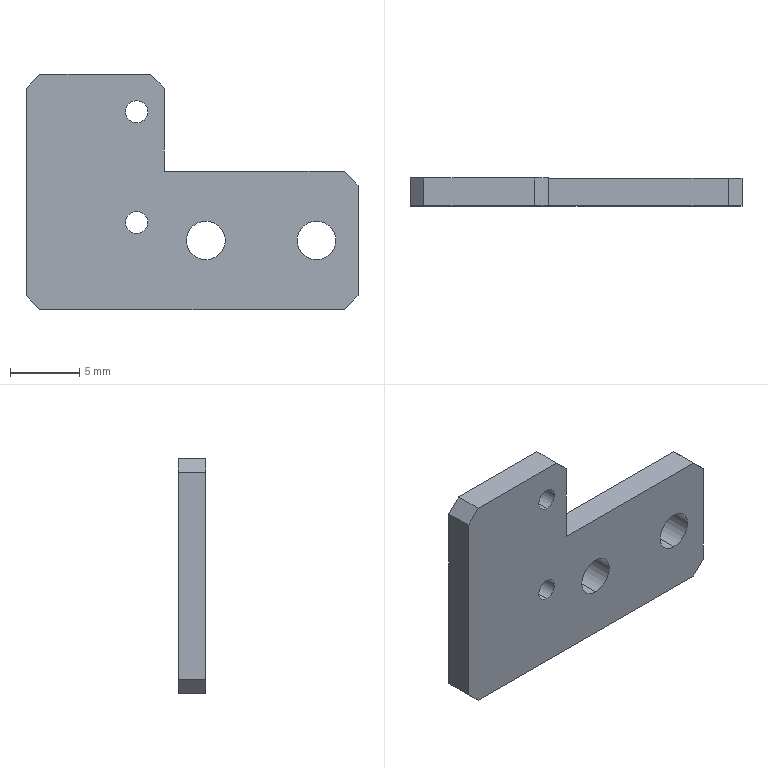Part | SolidWorks | features ICE 2, Chamfer 1, Extrusion 1, HoleWzd 1 | 1 solid | 21 faces | box 24 x 2 x 17 mm | volume 582.327 mm3 | plane 13 | cylinder 8 | commonest cylinder face diameters 1.6 x4 2.8 x4
STEP:
#1=CARTESIAN_POINT('',(8.,0.,-9.9));
#2=VERTEX_POINT('',#1);
#3=CARTESIAN_POINT('',(8.,0.,-11.5));
#4=VERTEX_POINT('',#3);
#5=CARTESIAN_POINT('',(8.,0.,-10.7));
#6=DIRECTION('',(0.,-1.,0.));
#7=DIRECTION('',(0.,0.,-1.));
#8=AXIS2_PLACEMENT_3D('',#5,#6,#7);
#9=CIRCLE('',#8,0.8);
#10=EDGE_CURVE('',#2,#4,#9,.T.);
#11=ORIENTED_EDGE('',*,*,#10,.T.);
#12=CARTESIAN_POINT('',(8.,2.,-11.5));
#13=VERTEX_POINT('',#12);
#14=CARTESIAN_POINT('',(8.,2.,-11.5));
#15=DIRECTION('',(0.,1.,0.));
#16=VECTOR('',#15,1000.);
#17=LINE('',#14,#16);
#18=EDGE_CURVE('',#4,#13,#17,.T.);
#19=ORIENTED_EDGE('',*,*,#18,.T.);
#20=CARTESIAN_POINT('',(8.,2.,-9.9));
#21=VERTEX_POINT('',#20);
#22=CARTESIAN_POINT('',(8.,2.,-10.7));
#23=DIRECTION('',(0.,1.,0.));
#24=DIRECTION('',(0.,0.,1.));
#25=AXIS2_PLACEMENT_3D('',#22,#23,#24);
#26=CIRCLE('',#25,0.8);
#27=EDGE_CURVE('',#13,#21,#26,.T.);
#28=ORIENTED_EDGE('',*,*,#27,.T.);
#29=CARTESIAN_POINT('',(8.,2.,-9.9));
#30=DIRECTION('',(0.,1.,0.));
#31=VECTOR('',#30,1000.);
#32=LINE('',#29,#31);
#33=EDGE_CURVE('',#2,#21,#32,.T.);
#34=ORIENTED_EDGE('',*,*,#33,.F.);
#35=EDGE_LOOP('',(#11,#19,#28,#34));
#36=FACE_OUTER_BOUND('',#35,.T.);
#37=CARTESIAN_POINT('',(8.,2.,-10.7));
#38=DIRECTION('',(0.,1.,0.));
#39=DIRECTION('',(0.,0.,1.));
#40=AXIS2_PLACEMENT_3D('',#37,#38,#39);
#41=CYLINDRICAL_SURFACE('',#40,0.8);
#42=ADVANCED_FACE('',(#36),#41,.F.);
#43=CARTESIAN_POINT('',(8.,0.,-1.9));
#44=VERTEX_POINT('',#43);
#45=CARTESIAN_POINT('',(8.,0.,-3.5));
#46=VERTEX_POINT('',#45);
#47=CARTESIAN_POINT('',(8.,0.,-2.7));
#48=DIRECTION('',(0.,-1.,0.));
#49=DIRECTION('',(0.,0.,-1.));
#50=AXIS2_PLACEMENT_3D('',#47,#48,#49);
#51=CIRCLE('',#50,0.8);
#52=EDGE_CURVE('',#44,#46,#51,.T.);
#53=ORIENTED_EDGE('',*,*,#52,.T.);
#54=CARTESIAN_POINT('',(8.,2.,-3.5));
#55=VERTEX_POINT('',#54);
#56=CARTESIAN_POINT('',(8.,2.,-3.5));
#57=DIRECTION('',(0.,1.,0.));
#58=VECTOR('',#57,1000.);
#59=LINE('',#56,#58);
#60=EDGE_CURVE('',#46,#55,#59,.T.);
#61=ORIENTED_EDGE('',*,*,#60,.T.);
#62=CARTESIAN_POINT('',(8.,2.,-1.9));
#63=VERTEX_POINT('',#62);
#64=CARTESIAN_POINT('',(8.,2.,-2.7));
#65=DIRECTION('',(0.,1.,0.));
#66=DIRECTION('',(0.,0.,1.));
#67=AXIS2_PLACEMENT_3D('',#64,#65,#66);
#68=CIRCLE('',#67,0.8);
#69=EDGE_CURVE('',#55,#63,#68,.T.);
#70=ORIENTED_EDGE('',*,*,#69,.T.);
#71=CARTESIAN_POINT('',(8.,2.,-1.9));
#72=DIRECTION('',(0.,1.,0.));
#73=VECTOR('',#72,1000.);
#74=LINE('',#71,#73);
#75=EDGE_CURVE('',#44,#63,#74,.T.);
#76=ORIENTED_EDGE('',*,*,#75,.F.);
#77=EDGE_LOOP('',(#53,#61,#70,#76));
#78=FACE_OUTER_BOUND('',#77,.T.);
#79=CARTESIAN_POINT('',(8.,2.,-2.7));
#80=DIRECTION('',(0.,1.,0.));
#81=DIRECTION('',(0.,0.,1.));
#82=AXIS2_PLACEMENT_3D('',#79,#80,#81);
#83=CYLINDRICAL_SURFACE('',#82,0.8);
#84=ADVANCED_FACE('',(#78),#83,.F.);
#85=CARTESIAN_POINT('',(13.,0.,-10.6));
#86=VERTEX_POINT('',#85);
#87=CARTESIAN_POINT('',(13.,0.,-13.4));
#88=VERTEX_POINT('',#87);
#89=CARTESIAN_POINT('',(13.,0.,-12.));
#90=DIRECTION('',(0.,-1.,0.));
#91=DIRECTION('',(0.,0.,-1.));
#92=AXIS2_PLACEMENT_3D('',#89,#90,#91);
#93=CIRCLE('',#92,1.4);
#94=EDGE_CURVE('',#86,#88,#93,.T.);
#95=ORIENTED_EDGE('',*,*,#94,.T.);
#96=CARTESIAN_POINT('',(13.,2.,-13.4));
#97=VERTEX_POINT('',#96);
#98=CARTESIAN_POINT('',(13.,-8.,-13.4));
#99=DIRECTION('',(0.,1.,0.));
#100=VECTOR('',#99,1000.);
#101=LINE('',#98,#100);
#102=EDGE_CURVE('',#88,#97,#101,.T.);
#103=ORIENTED_EDGE('',*,*,#102,.T.);
#104=CARTESIAN_POINT('',(13.,2.,-10.6));
#105=VERTEX_POINT('',#104);
#106=CARTESIAN_POINT('',(13.,2.,-12.));
#107=DIRECTION('',(0.,1.,0.));
#108=DIRECTION('',(0.,0.,1.));
#109=AXIS2_PLACEMENT_3D('',#106,#107,#108);
#110=CIRCLE('',#109,1.4);
#111=EDGE_CURVE('',#97,#105,#110,.T.);
#112=ORIENTED_EDGE('',*,*,#111,.T.);
#113=CARTESIAN_POINT('',(13.,-8.,-10.6));
#114=DIRECTION('',(0.,1.,0.));
#115=VECTOR('',#114,1000.);
#116=LINE('',#113,#115);
#117=EDGE_CURVE('',#86,#105,#116,.T.);
#118=ORIENTED_EDGE('',*,*,#117,.F.);
#119=EDGE_LOOP('',(#95,#103,#112,#118));
#120=FACE_OUTER_BOUND('',#119,.T.);
#121=CARTESIAN_POINT('',(13.,-8.,-12.));
#122=DIRECTION('',(0.,1.,0.));
#123=DIRECTION('',(0.,0.,1.));
#124=AXIS2_PLACEMENT_3D('',#121,#122,#123);
#125=CYLINDRICAL_SURFACE('',#124,1.4);
#126=ADVANCED_FACE('',(#120),#125,.F.);
#127=CARTESIAN_POINT('',(21.,0.,-10.6));
#128=VERTEX_POINT('',#127);
#129=CARTESIAN_POINT('',(21.,0.,-13.4));
#130=VERTEX_POINT('',#129);
#131=CARTESIAN_POINT('',(21.,0.,-12.));
#132=DIRECTION('',(0.,-1.,0.));
#133=DIRECTION('',(0.,0.,-1.));
#134=AXIS2_PLACEMENT_3D('',#131,#132,#133);
#135=CIRCLE('',#134,1.4);
#136=EDGE_CURVE('',#128,#130,#135,.T.);
#137=ORIENTED_EDGE('',*,*,#136,.T.);
#138=CARTESIAN_POINT('',(21.,2.,-13.4));
#139=VERTEX_POINT('',#138);
#140=CARTESIAN_POINT('',(21.,-8.,-13.4));
#141=DIRECTION('',(0.,1.,0.));
#142=VECTOR('',#141,1000.);
#143=LINE('',#140,#142);
#144=EDGE_CURVE('',#130,#139,#143,.T.);
#145=ORIENTED_EDGE('',*,*,#144,.T.);
#146=CARTESIAN_POINT('',(21.,2.,-10.6));
#147=VERTEX_POINT('',#146);
#148=CARTESIAN_POINT('',(21.,2.,-12.));
#149=DIRECTION('',(0.,1.,0.));
#150=DIRECTION('',(0.,0.,1.));
#151=AXIS2_PLACEMENT_3D('',#148,#149,#150);
#152=CIRCLE('',#151,1.4);
#153=EDGE_CURVE('',#139,#147,#152,.T.);
#154=ORIENTED_EDGE('',*,*,#153,.T.);
#155=CARTESIAN_POINT('',(21.,-8.,-10.6));
#156=DIRECTION('',(0.,1.,0.));
#157=VECTOR('',#156,1000.);
#158=LINE('',#155,#157);
#159=EDGE_CURVE('',#128,#147,#158,.T.);
#160=ORIENTED_EDGE('',*,*,#159,.F.);
#161=EDGE_LOOP('',(#137,#145,#154,#160));
#162=FACE_OUTER_BOUND('',#161,.T.);
#163=CARTESIAN_POINT('',(21.,-8.,-12.));
#164=DIRECTION('',(0.,1.,0.));
#165=DIRECTION('',(0.,0.,1.));
#166=AXIS2_PLACEMENT_3D('',#163,#164,#165);
#167=CYLINDRICAL_SURFACE('',#166,1.4);
#168=ADVANCED_FACE('',(#162),#167,.F.);
#169=CARTESIAN_POINT('',(0.,2.,-16.));
#170=VERTEX_POINT('',#169);
#171=CARTESIAN_POINT('',(0.,2.,-1.));
#172=VERTEX_POINT('',#171);
#173=CARTESIAN_POINT('',(0.,2.,0.));
#174=DIRECTION('',(0.,0.,1.));
#175=VECTOR('',#174,1000.);
#176=LINE('',#173,#175);
#177=EDGE_CURVE('',#170,#172,#176,.T.);
#178=ORIENTED_EDGE('',*,*,#177,.F.);
#179=CARTESIAN_POINT('',(0.,0.,-16.));
#180=VERTEX_POINT('',#179);
#181=CARTESIAN_POINT('',(0.,2.,-16.));
#182=DIRECTION('',(0.,-1.,0.));
#183=VECTOR('',#182,1000.);
#184=LINE('',#181,#183);
#185=EDGE_CURVE('',#170,#180,#184,.T.);
#186=ORIENTED_EDGE('',*,*,#185,.T.);
#187=CARTESIAN_POINT('',(0.,0.,-1.));
#188=VERTEX_POINT('',#187);
#189=CARTESIAN_POINT('',(0.,0.,0.));
#190=DIRECTION('',(0.,0.,1.));
#191=VECTOR('',#190,1000.);
#192=LINE('',#189,#191);
#193=EDGE_CURVE('',#180,#188,#192,.T.);
#194=ORIENTED_EDGE('',*,*,#193,.T.);
#195=CARTESIAN_POINT('',(0.,2.,-1.));
#196=DIRECTION('',(0.,1.,0.));
#197=VECTOR('',#196,1000.);
#198=LINE('',#195,#197);
#199=EDGE_CURVE('',#188,#172,#198,.T.);
#200=ORIENTED_EDGE('',*,*,#199,.T.);
#201=EDGE_LOOP('',(#178,#186,#194,#200));
#202=FACE_OUTER_BOUND('',#201,.T.);
#203=CARTESIAN_POINT('',(0.,2.,0.));
#204=DIRECTION('',(1.,0.,0.));
#205=DIRECTION('',(0.,0.,-1.));
#206=AXIS2_PLACEMENT_3D('',#203,#204,#205);
#207=PLANE('',#206);
#208=ADVANCED_FACE('',(#202),#207,.F.);
#209=CARTESIAN_POINT('',(1.,2.,0.));
#210=VERTEX_POINT('',#209);
#211=CARTESIAN_POINT('',(9.,2.,0.));
#212=VERTEX_POINT('',#211);
#213=CARTESIAN_POINT('',(0.,2.,0.));
#214=DIRECTION('',(1.,0.,0.));
#215=VECTOR('',#214,1000.);
#216=LINE('',#213,#215);
#217=EDGE_CURVE('',#210,#212,#216,.T.);
#218=ORIENTED_EDGE('',*,*,#217,.F.);
#219=CARTESIAN_POINT('',(1.,0.,0.));
#220=VERTEX_POINT('',#219);
#221=CARTESIAN_POINT('',(1.,2.,0.));
#222=DIRECTION('',(0.,-1.,0.));
#223=VECTOR('',#222,1000.);
#224=LINE('',#221,#223);
#225=EDGE_CURVE('',#210,#220,#224,.T.);
#226=ORIENTED_EDGE('',*,*,#225,.T.);
#227=CARTESIAN_POINT('',(9.,0.,0.));
#228=VERTEX_POINT('',#227);
#229=CARTESIAN_POINT('',(0.,0.,0.));
#230=DIRECTION('',(1.,0.,0.));
#231=VECTOR('',#230,1000.);
#232=LINE('',#229,#231);
#233=EDGE_CURVE('',#220,#228,#232,.T.);
#234=ORIENTED_EDGE('',*,*,#233,.T.);
#235=CARTESIAN_POINT('',(9.,2.,0.));
#236=DIRECTION('',(0.,1.,0.));
#237=VECTOR('',#236,1000.);
#238=LINE('',#235,#237);
#239=EDGE_CURVE('',#228,#212,#238,.T.);
#240=ORIENTED_EDGE('',*,*,#239,.T.);
#241=EDGE_LOOP('',(#218,#226,#234,#240));
#242=FACE_OUTER_BOUND('',#241,.T.);
#243=CARTESIAN_POINT('',(0.,2.,0.));
#244=DIRECTION('',(0.,0.,-1.));
#245=DIRECTION('',(-1.,0.,0.));
#246=AXIS2_PLACEMENT_3D('',#243,#244,#245);
#247=PLANE('',#246);
#248=ADVANCED_FACE('',(#242),#247,.F.);
#249=CARTESIAN_POINT('',(10.,2.,-1.));
#250=VERTEX_POINT('',#249);
#251=CARTESIAN_POINT('',(10.,2.,-7.));
#252=VERTEX_POINT('',#251);
#253=CARTESIAN_POINT('',(10.,2.,0.));
#254=DIRECTION('',(0.,0.,-1.));
#255=VECTOR('',#254,1000.);
#256=LINE('',#253,#255);
#257=EDGE_CURVE('',#250,#252,#256,.T.);
#258=ORIENTED_EDGE('',*,*,#257,.F.);
#259=CARTESIAN_POINT('',(10.,0.,-1.));
#260=VERTEX_POINT('',#259);
#261=CARTESIAN_POINT('',(10.,2.,-1.));
#262=DIRECTION('',(0.,-1.,0.));
#263=VECTOR('',#262,1000.);
#264=LINE('',#261,#263);
#265=EDGE_CURVE('',#250,#260,#264,.T.);
#266=ORIENTED_EDGE('',*,*,#265,.T.);
#267=CARTESIAN_POINT('',(10.,0.,-7.));
#268=VERTEX_POINT('',#267);
#269=CARTESIAN_POINT('',(10.,0.,0.));
#270=DIRECTION('',(0.,0.,-1.));
#271=VECTOR('',#270,1000.);
#272=LINE('',#269,#271);
#273=EDGE_CURVE('',#260,#268,#272,.T.);
#274=ORIENTED_EDGE('',*,*,#273,.T.);
#275=CARTESIAN_POINT('',(10.,0.,-7.));
#276=DIRECTION('',(0.,1.,0.));
#277=VECTOR('',#276,1000.);
#278=LINE('',#275,#277);
#279=EDGE_CURVE('',#268,#252,#278,.T.);
#280=ORIENTED_EDGE('',*,*,#279,.T.);
#281=EDGE_LOOP('',(#258,#266,#274,#280));
#282=FACE_OUTER_BOUND('',#281,.T.);
#283=CARTESIAN_POINT('',(10.,2.,0.));
#284=DIRECTION('',(-1.,0.,0.));
#285=DIRECTION('',(0.,0.,1.));
#286=AXIS2_PLACEMENT_3D('',#283,#284,#285);
#287=PLANE('',#286);
#288=ADVANCED_FACE('',(#282),#287,.F.);
#289=CARTESIAN_POINT('',(23.,0.,-17.));
#290=VERTEX_POINT('',#289);
#291=CARTESIAN_POINT('',(1.,0.,-17.));
#292=VERTEX_POINT('',#291);
#293=CARTESIAN_POINT('',(0.,0.,-17.));
#294=DIRECTION('',(-1.,0.,0.));
#295=VECTOR('',#294,1000.);
#296=LINE('',#293,#295);
#297=EDGE_CURVE('',#290,#292,#296,.T.);
#298=ORIENTED_EDGE('',*,*,#297,.T.);
#299=CARTESIAN_POINT('',(1.,2.,-17.));
#300=VERTEX_POINT('',#299);
#301=CARTESIAN_POINT('',(1.,2.,-17.));
#302=DIRECTION('',(0.,1.,0.));
#303=VECTOR('',#302,1000.);
#304=LINE('',#301,#303);
#305=EDGE_CURVE('',#292,#300,#304,.T.);
#306=ORIENTED_EDGE('',*,*,#305,.T.);
#307=CARTESIAN_POINT('',(23.,2.,-17.));
#308=VERTEX_POINT('',#307);
#309=CARTESIAN_POINT('',(0.,2.,-17.));
#310=DIRECTION('',(-1.,0.,0.));
#311=VECTOR('',#310,1000.);
#312=LINE('',#309,#311);
#313=EDGE_CURVE('',#308,#300,#312,.T.);
#314=ORIENTED_EDGE('',*,*,#313,.F.);
#315=CARTESIAN_POINT('',(23.,0.,-17.));
#316=DIRECTION('',(0.,-1.,0.));
#317=VECTOR('',#316,1000.);
#318=LINE('',#315,#317);
#319=EDGE_CURVE('',#308,#290,#318,.T.);
#320=ORIENTED_EDGE('',*,*,#319,.T.);
#321=EDGE_LOOP('',(#298,#306,#314,#320));
#322=FACE_OUTER_BOUND('',#321,.T.);
#323=CARTESIAN_POINT('',(0.,2.,-17.));
#324=DIRECTION('',(0.,0.,1.));
#325=DIRECTION('',(1.,0.,0.));
#326=AXIS2_PLACEMENT_3D('',#323,#324,#325);
#327=PLANE('',#326);
#328=ADVANCED_FACE('',(#322),#327,.F.);
#329=CARTESIAN_POINT('',(8.,2.,-10.7));
#330=DIRECTION('',(0.,1.,0.));
#331=DIRECTION('',(0.,0.,1.));
#332=AXIS2_PLACEMENT_3D('',#329,#330,#331);
#333=CIRCLE('',#332,0.8);
#334=EDGE_CURVE('',#21,#13,#333,.T.);
#335=ORIENTED_EDGE('',*,*,#334,.F.);
#336=ORIENTED_EDGE('',*,*,#27,.F.);
#337=EDGE_LOOP('',(#335,#336));
#338=FACE_BOUND('',#337,.T.);
#339=CARTESIAN_POINT('',(8.,2.,-2.7));
#340=DIRECTION('',(0.,1.,0.));
#341=DIRECTION('',(0.,0.,1.));
#342=AXIS2_PLACEMENT_3D('',#339,#340,#341);
#343=CIRCLE('',#342,0.8);
#344=EDGE_CURVE('',#63,#55,#343,.T.);
#345=ORIENTED_EDGE('',*,*,#344,.F.);
#346=ORIENTED_EDGE('',*,*,#69,.F.);
#347=EDGE_LOOP('',(#345,#346));
#348=FACE_BOUND('',#347,.T.);
#349=CARTESIAN_POINT('',(13.,2.,-12.));
#350=DIRECTION('',(0.,1.,0.));
#351=DIRECTION('',(0.,0.,1.));
#352=AXIS2_PLACEMENT_3D('',#349,#350,#351);
#353=CIRCLE('',#352,1.4);
#354=EDGE_CURVE('',#105,#97,#353,.T.);
#355=ORIENTED_EDGE('',*,*,#354,.F.);
#356=ORIENTED_EDGE('',*,*,#111,.F.);
#357=EDGE_LOOP('',(#355,#356));
#358=FACE_BOUND('',#357,.T.);
#359=CARTESIAN_POINT('',(21.,2.,-12.));
#360=DIRECTION('',(0.,1.,0.));
#361=DIRECTION('',(0.,0.,1.));
#362=AXIS2_PLACEMENT_3D('',#359,#360,#361);
#363=CIRCLE('',#362,1.4);
#364=EDGE_CURVE('',#147,#139,#363,.T.);
#365=ORIENTED_EDGE('',*,*,#364,.F.);
#366=ORIENTED_EDGE('',*,*,#153,.F.);
#367=EDGE_LOOP('',(#365,#366));
#368=FACE_BOUND('',#367,.T.);
#369=ORIENTED_EDGE('',*,*,#313,.T.);
#370=CARTESIAN_POINT('',(0.,2.,-16.));
#371=DIRECTION('',(-0.7071,0.,0.7071));
#372=VECTOR('',#371,1000.);
#373=LINE('',#370,#372);
#374=EDGE_CURVE('',#300,#170,#373,.T.);
#375=ORIENTED_EDGE('',*,*,#374,.T.);
#376=ORIENTED_EDGE('',*,*,#177,.T.);
#377=CARTESIAN_POINT('',(1.,2.,0.));
#378=DIRECTION('',(0.7071,0.,0.7071));
#379=VECTOR('',#378,1000.);
#380=LINE('',#377,#379);
#381=EDGE_CURVE('',#172,#210,#380,.T.);
#382=ORIENTED_EDGE('',*,*,#381,.T.);
#383=ORIENTED_EDGE('',*,*,#217,.T.);
#384=CARTESIAN_POINT('',(10.,2.,-1.));
#385=DIRECTION('',(0.7071,0.,-0.7071));
#386=VECTOR('',#385,1000.);
#387=LINE('',#384,#386);
#388=EDGE_CURVE('',#212,#250,#387,.T.);
#389=ORIENTED_EDGE('',*,*,#388,.T.);
#390=ORIENTED_EDGE('',*,*,#257,.T.);
#391=CARTESIAN_POINT('',(23.,2.,-7.));
#392=VERTEX_POINT('',#391);
#393=CARTESIAN_POINT('',(10.,2.,-7.));
#394=DIRECTION('',(1.,0.,0.));
#395=VECTOR('',#394,1000.);
#396=LINE('',#393,#395);
#397=EDGE_CURVE('',#252,#392,#396,.T.);
#398=ORIENTED_EDGE('',*,*,#397,.T.);
#399=CARTESIAN_POINT('',(24.,2.,-8.));
#400=VERTEX_POINT('',#399);
#401=CARTESIAN_POINT('',(23.,2.,-7.));
#402=DIRECTION('',(0.7071,0.,-0.7071));
#403=VECTOR('',#402,1000.);
#404=LINE('',#401,#403);
#405=EDGE_CURVE('',#392,#400,#404,.T.);
#406=ORIENTED_EDGE('',*,*,#405,.T.);
#407=CARTESIAN_POINT('',(24.,2.,-16.));
#408=VERTEX_POINT('',#407);
#409=CARTESIAN_POINT('',(24.,2.,-17.));
#410=DIRECTION('',(0.,0.,-1.));
#411=VECTOR('',#410,1000.);
#412=LINE('',#409,#411);
#413=EDGE_CURVE('',#400,#408,#412,.T.);
#414=ORIENTED_EDGE('',*,*,#413,.T.);
#415=CARTESIAN_POINT('',(24.,2.,-16.));
#416=DIRECTION('',(-0.7071,0.,-0.7071));
#417=VECTOR('',#416,1000.);
#418=LINE('',#415,#417);
#419=EDGE_CURVE('',#408,#308,#418,.T.);
#420=ORIENTED_EDGE('',*,*,#419,.T.);
#421=EDGE_LOOP('',(#369,#375,#376,#382,#383,#389,#390,#398,#406,#414,#420));
#422=FACE_OUTER_BOUND('',#421,.T.);
#423=CARTESIAN_POINT('',(0.,2.,0.));
#424=DIRECTION('',(0.,-1.,0.));
#425=DIRECTION('',(0.,0.,-1.));
#426=AXIS2_PLACEMENT_3D('',#423,#424,#425);
#427=PLANE('',#426);
#428=ADVANCED_FACE('',(#338,#348,#358,#368,#422),#427,.F.);
#429=ORIENTED_EDGE('',*,*,#10,.F.);
#430=CARTESIAN_POINT('',(8.,0.,-10.7));
#431=DIRECTION('',(0.,-1.,0.));
#432=DIRECTION('',(0.,0.,-1.));
#433=AXIS2_PLACEMENT_3D('',#430,#431,#432);
#434=CIRCLE('',#433,0.8);
#435=EDGE_CURVE('',#4,#2,#434,.T.);
#436=ORIENTED_EDGE('',*,*,#435,.F.);
#437=EDGE_LOOP('',(#429,#436));
#438=FACE_BOUND('',#437,.T.);
#439=ORIENTED_EDGE('',*,*,#52,.F.);
#440=CARTESIAN_POINT('',(8.,0.,-2.7));
#441=DIRECTION('',(0.,-1.,0.));
#442=DIRECTION('',(0.,0.,-1.));
#443=AXIS2_PLACEMENT_3D('',#440,#441,#442);
#444=CIRCLE('',#443,0.8);
#445=EDGE_CURVE('',#46,#44,#444,.T.);
#446=ORIENTED_EDGE('',*,*,#445,.F.);
#447=EDGE_LOOP('',(#439,#446));
#448=FACE_BOUND('',#447,.T.);
#449=ORIENTED_EDGE('',*,*,#94,.F.);
#450=CARTESIAN_POINT('',(13.,0.,-12.));
#451=DIRECTION('',(0.,-1.,0.));
#452=DIRECTION('',(0.,0.,-1.));
#453=AXIS2_PLACEMENT_3D('',#450,#451,#452);
#454=CIRCLE('',#453,1.4);
#455=EDGE_CURVE('',#88,#86,#454,.T.);
#456=ORIENTED_EDGE('',*,*,#455,.F.);
#457=EDGE_LOOP('',(#449,#456));
#458=FACE_BOUND('',#457,.T.);
#459=ORIENTED_EDGE('',*,*,#136,.F.);
#460=CARTESIAN_POINT('',(21.,0.,-12.));
#461=DIRECTION('',(0.,-1.,0.));
#462=DIRECTION('',(0.,0.,-1.));
#463=AXIS2_PLACEMENT_3D('',#460,#461,#462);
#464=CIRCLE('',#463,1.4);
#465=EDGE_CURVE('',#130,#128,#464,.T.);
#466=ORIENTED_EDGE('',*,*,#465,.F.);
#467=EDGE_LOOP('',(#459,#466));
#468=FACE_BOUND('',#467,.T.);
#469=ORIENTED_EDGE('',*,*,#193,.F.);
#470=CARTESIAN_POINT('',(-8.,0.,-8.));
#471=DIRECTION('',(0.7071,0.,-0.7071));
#472=VECTOR('',#471,1000.);
#473=LINE('',#470,#472);
#474=EDGE_CURVE('',#180,#292,#473,.T.);
#475=ORIENTED_EDGE('',*,*,#474,.T.);
#476=ORIENTED_EDGE('',*,*,#297,.F.);
#477=CARTESIAN_POINT('',(24.,0.,-16.));
#478=VERTEX_POINT('',#477);
#479=CARTESIAN_POINT('',(20.,0.,-20.));
#480=DIRECTION('',(0.7071,0.,0.7071));
#481=VECTOR('',#480,1000.);
#482=LINE('',#479,#481);
#483=EDGE_CURVE('',#290,#478,#482,.T.);
#484=ORIENTED_EDGE('',*,*,#483,.T.);
#485=CARTESIAN_POINT('',(24.,0.,-8.));
#486=VERTEX_POINT('',#485);
#487=CARTESIAN_POINT('',(24.,0.,-17.));
#488=DIRECTION('',(0.,0.,-1.));
#489=VECTOR('',#488,1000.);
#490=LINE('',#487,#489);
#491=EDGE_CURVE('',#486,#478,#490,.T.);
#492=ORIENTED_EDGE('',*,*,#491,.F.);
#493=CARTESIAN_POINT('',(23.,0.,-7.));
#494=VERTEX_POINT('',#493);
#495=CARTESIAN_POINT('',(8.,0.,8.));
#496=DIRECTION('',(-0.7071,0.,0.7071));
#497=VECTOR('',#496,1000.);
#498=LINE('',#495,#497);
#499=EDGE_CURVE('',#486,#494,#498,.T.);
#500=ORIENTED_EDGE('',*,*,#499,.T.);
#501=CARTESIAN_POINT('',(10.,0.,-7.));
#502=DIRECTION('',(1.,0.,0.));
#503=VECTOR('',#502,1000.);
#504=LINE('',#501,#503);
#505=EDGE_CURVE('',#268,#494,#504,.T.);
#506=ORIENTED_EDGE('',*,*,#505,.F.);
#507=ORIENTED_EDGE('',*,*,#273,.F.);
#508=CARTESIAN_POINT('',(4.5,0.,4.5));
#509=DIRECTION('',(-0.7071,0.,0.7071));
#510=VECTOR('',#509,1000.);
#511=LINE('',#508,#510);
#512=EDGE_CURVE('',#260,#228,#511,.T.);
#513=ORIENTED_EDGE('',*,*,#512,.T.);
#514=ORIENTED_EDGE('',*,*,#233,.F.);
#515=CARTESIAN_POINT('',(0.5,0.,-0.5));
#516=DIRECTION('',(-0.7071,0.,-0.7071));
#517=VECTOR('',#516,1000.);
#518=LINE('',#515,#517);
#519=EDGE_CURVE('',#220,#188,#518,.T.);
#520=ORIENTED_EDGE('',*,*,#519,.T.);
#521=EDGE_LOOP('',(#469,#475,#476,#484,#492,#500,#506,#507,#513,#514,#520));
#522=FACE_OUTER_BOUND('',#521,.T.);
#523=CARTESIAN_POINT('',(0.,0.,0.));
#524=DIRECTION('',(0.,-1.,0.));
#525=DIRECTION('',(0.,0.,-1.));
#526=AXIS2_PLACEMENT_3D('',#523,#524,#525);
#527=PLANE('',#526);
#528=ADVANCED_FACE('',(#438,#448,#458,#468,#522),#527,.T.);
#529=ORIENTED_EDGE('',*,*,#491,.T.);
#530=CARTESIAN_POINT('',(24.,2.,-16.));
#531=DIRECTION('',(0.,1.,0.));
#532=VECTOR('',#531,1000.);
#533=LINE('',#530,#532);
#534=EDGE_CURVE('',#478,#408,#533,.T.);
#535=ORIENTED_EDGE('',*,*,#534,.T.);
#536=ORIENTED_EDGE('',*,*,#413,.F.);
#537=CARTESIAN_POINT('',(24.,0.,-8.));
#538=DIRECTION('',(0.,-1.,0.));
#539=VECTOR('',#538,1000.);
#540=LINE('',#537,#539);
#541=EDGE_CURVE('',#400,#486,#540,.T.);
#542=ORIENTED_EDGE('',*,*,#541,.T.);
#543=EDGE_LOOP('',(#529,#535,#536,#542));
#544=FACE_OUTER_BOUND('',#543,.T.);
#545=CARTESIAN_POINT('',(24.,0.,-17.));
#546=DIRECTION('',(1.,0.,0.));
#547=DIRECTION('',(0.,0.,-1.));
#548=AXIS2_PLACEMENT_3D('',#545,#546,#547);
#549=PLANE('',#548);
#550=ADVANCED_FACE('',(#544),#549,.T.);
#551=ORIENTED_EDGE('',*,*,#505,.T.);
#552=CARTESIAN_POINT('',(23.,0.,-7.));
#553=DIRECTION('',(0.,1.,0.));
#554=VECTOR('',#553,1000.);
#555=LINE('',#552,#554);
#556=EDGE_CURVE('',#494,#392,#555,.T.);
#557=ORIENTED_EDGE('',*,*,#556,.T.);
#558=ORIENTED_EDGE('',*,*,#397,.F.);
#559=ORIENTED_EDGE('',*,*,#279,.F.);
#560=EDGE_LOOP('',(#551,#557,#558,#559));
#561=FACE_OUTER_BOUND('',#560,.T.);
#562=CARTESIAN_POINT('',(10.,0.,-7.));
#563=DIRECTION('',(0.,0.,1.));
#564=DIRECTION('',(1.,0.,0.));
#565=AXIS2_PLACEMENT_3D('',#562,#563,#564);
#566=PLANE('',#565);
#567=ADVANCED_FACE('',(#561),#566,.T.);
#568=ORIENTED_EDGE('',*,*,#144,.F.);
#569=ORIENTED_EDGE('',*,*,#465,.T.);
#570=ORIENTED_EDGE('',*,*,#159,.T.);
#571=ORIENTED_EDGE('',*,*,#364,.T.);
#572=EDGE_LOOP('',(#568,#569,#570,#571));
#573=FACE_OUTER_BOUND('',#572,.T.);
#574=CARTESIAN_POINT('',(21.,-8.,-12.));
#575=DIRECTION('',(0.,1.,0.));
#576=DIRECTION('',(0.,0.,1.));
#577=AXIS2_PLACEMENT_3D('',#574,#575,#576);
#578=CYLINDRICAL_SURFACE('',#577,1.4);
#579=ADVANCED_FACE('',(#573),#578,.F.);
#580=ORIENTED_EDGE('',*,*,#102,.F.);
#581=ORIENTED_EDGE('',*,*,#455,.T.);
#582=ORIENTED_EDGE('',*,*,#117,.T.);
#583=ORIENTED_EDGE('',*,*,#354,.T.);
#584=EDGE_LOOP('',(#580,#581,#582,#583));
#585=FACE_OUTER_BOUND('',#584,.T.);
#586=CARTESIAN_POINT('',(13.,-8.,-12.));
#587=DIRECTION('',(0.,1.,0.));
#588=DIRECTION('',(0.,0.,1.));
#589=AXIS2_PLACEMENT_3D('',#586,#587,#588);
#590=CYLINDRICAL_SURFACE('',#589,1.4);
#591=ADVANCED_FACE('',(#585),#590,.F.);
#592=ORIENTED_EDGE('',*,*,#374,.F.);
#593=ORIENTED_EDGE('',*,*,#305,.F.);
#594=ORIENTED_EDGE('',*,*,#474,.F.);
#595=ORIENTED_EDGE('',*,*,#185,.F.);
#596=EDGE_LOOP('',(#592,#593,#594,#595));
#597=FACE_OUTER_BOUND('',#596,.T.);
#598=CARTESIAN_POINT('',(0.,2.,-16.));
#599=DIRECTION('',(0.7071,0.,0.7071));
#600=DIRECTION('',(0.,-1.,0.));
#601=AXIS2_PLACEMENT_3D('',#598,#599,#600);
#602=PLANE('',#601);
#603=ADVANCED_FACE('',(#597),#602,.F.);
#604=ORIENTED_EDGE('',*,*,#381,.F.);
#605=ORIENTED_EDGE('',*,*,#199,.F.);
#606=ORIENTED_EDGE('',*,*,#519,.F.);
#607=ORIENTED_EDGE('',*,*,#225,.F.);
#608=EDGE_LOOP('',(#604,#605,#606,#607));
#609=FACE_OUTER_BOUND('',#608,.T.);
#610=CARTESIAN_POINT('',(1.,2.,0.));
#611=DIRECTION('',(0.7071,0.,-0.7071));
#612=DIRECTION('',(0.,-1.,0.));
#613=AXIS2_PLACEMENT_3D('',#610,#611,#612);
#614=PLANE('',#613);
#615=ADVANCED_FACE('',(#609),#614,.F.);
#616=ORIENTED_EDGE('',*,*,#388,.F.);
#617=ORIENTED_EDGE('',*,*,#239,.F.);
#618=ORIENTED_EDGE('',*,*,#512,.F.);
#619=ORIENTED_EDGE('',*,*,#265,.F.);
#620=EDGE_LOOP('',(#616,#617,#618,#619));
#621=FACE_OUTER_BOUND('',#620,.T.);
#622=CARTESIAN_POINT('',(10.,2.,-1.));
#623=DIRECTION('',(-0.7071,0.,-0.7071));
#624=DIRECTION('',(0.,-1.,0.));
#625=AXIS2_PLACEMENT_3D('',#622,#623,#624);
#626=PLANE('',#625);
#627=ADVANCED_FACE('',(#621),#626,.F.);
#628=ORIENTED_EDGE('',*,*,#483,.F.);
#629=ORIENTED_EDGE('',*,*,#319,.F.);
#630=ORIENTED_EDGE('',*,*,#419,.F.);
#631=ORIENTED_EDGE('',*,*,#534,.F.);
#632=EDGE_LOOP('',(#628,#629,#630,#631));
#633=FACE_OUTER_BOUND('',#632,.T.);
#634=CARTESIAN_POINT('',(24.,0.,-16.));
#635=DIRECTION('',(0.7071,0.,-0.7071));
#636=DIRECTION('',(0.,-1.,0.));
#637=AXIS2_PLACEMENT_3D('',#634,#635,#636);
#638=PLANE('',#637);
#639=ADVANCED_FACE('',(#633),#638,.T.);
#640=ORIENTED_EDGE('',*,*,#499,.F.);
#641=ORIENTED_EDGE('',*,*,#541,.F.);
#642=ORIENTED_EDGE('',*,*,#405,.F.);
#643=ORIENTED_EDGE('',*,*,#556,.F.);
#644=EDGE_LOOP('',(#640,#641,#642,#643));
#645=FACE_OUTER_BOUND('',#644,.T.);
#646=CARTESIAN_POINT('',(23.,0.,-7.));
#647=DIRECTION('',(-0.7071,0.,-0.7071));
#648=DIRECTION('',(0.,1.,0.));
#649=AXIS2_PLACEMENT_3D('',#646,#647,#648);
#650=PLANE('',#649);
#651=ADVANCED_FACE('',(#645),#650,.F.);
#652=ORIENTED_EDGE('',*,*,#60,.F.);
#653=ORIENTED_EDGE('',*,*,#445,.T.);
#654=ORIENTED_EDGE('',*,*,#75,.T.);
#655=ORIENTED_EDGE('',*,*,#344,.T.);
#656=EDGE_LOOP('',(#652,#653,#654,#655));
#657=FACE_OUTER_BOUND('',#656,.T.);
#658=CARTESIAN_POINT('',(8.,2.,-2.7));
#659=DIRECTION('',(0.,1.,0.));
#660=DIRECTION('',(0.,0.,1.));
#661=AXIS2_PLACEMENT_3D('',#658,#659,#660);
#662=CYLINDRICAL_SURFACE('',#661,0.8);
#663=ADVANCED_FACE('',(#657),#662,.F.);
#664=ORIENTED_EDGE('',*,*,#18,.F.);
#665=ORIENTED_EDGE('',*,*,#435,.T.);
#666=ORIENTED_EDGE('',*,*,#33,.T.);
#667=ORIENTED_EDGE('',*,*,#334,.T.);
#668=EDGE_LOOP('',(#664,#665,#666,#667));
#669=FACE_OUTER_BOUND('',#668,.T.);
#670=CARTESIAN_POINT('',(8.,2.,-10.7));
#671=DIRECTION('',(0.,1.,0.));
#672=DIRECTION('',(0.,0.,1.));
#673=AXIS2_PLACEMENT_3D('',#670,#671,#672);
#674=CYLINDRICAL_SURFACE('',#673,0.8);
#675=ADVANCED_FACE('',(#669),#674,.F.);
#676=CLOSED_SHELL('',(#42,#84,#126,#168,#208,#248,#288,#328,#428,#528,#550,#567,#579,#591,#603,#615,#627,#639,#651,#663,#675));
#677=MANIFOLD_SOLID_BREP('',#676);
#678=CARTESIAN_POINT('',(0.,0.,0.));
#679=DIRECTION('',(0.,0.,1.));
#680=DIRECTION('',(1.,0.,0.));
#681=AXIS2_PLACEMENT_3D('',#678,#679,#680);
#682=(LENGTH_UNIT()NAMED_UNIT(*)SI_UNIT(.MILLI.,.METRE.));
#683=UNCERTAINTY_MEASURE_WITH_UNIT(LENGTH_MEASURE(0.00001),#682,'','');
#684=(NAMED_UNIT(*)PLANE_ANGLE_UNIT()SI_UNIT($,.RADIAN.));
#685=(NAMED_UNIT(*)SI_UNIT($,.STERADIAN.)SOLID_ANGLE_UNIT());
#686=(GEOMETRIC_REPRESENTATION_CONTEXT(3)GLOBAL_UNCERTAINTY_ASSIGNED_CONTEXT((#683))GLOBAL_UNIT_ASSIGNED_CONTEXT((#682,#684,#685))REPRESENTATION_CONTEXT('',''));
#687=ADVANCED_BREP_SHAPE_REPRESENTATION('',(#677,#681),#686);